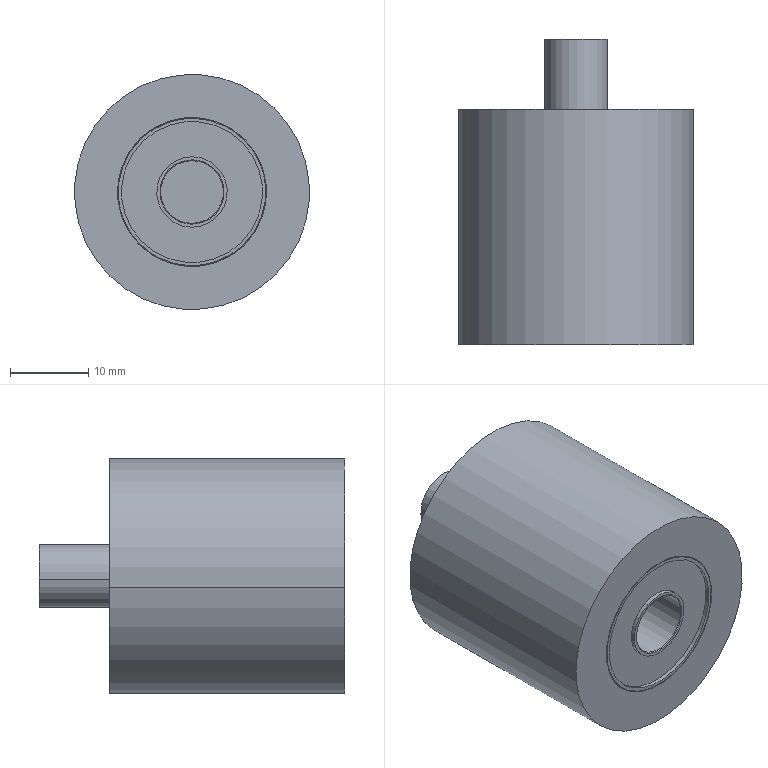Part | SolidWorks | 2 solids | 68 faces | box 30 x 39 x 30 mm | volume 17492 mm3 | cylinder 34 | plane 18 | spline 16 | commonest cylinder face diameters 9 x8 18 x8 19 x8 8 x6 15 x2 30 x2